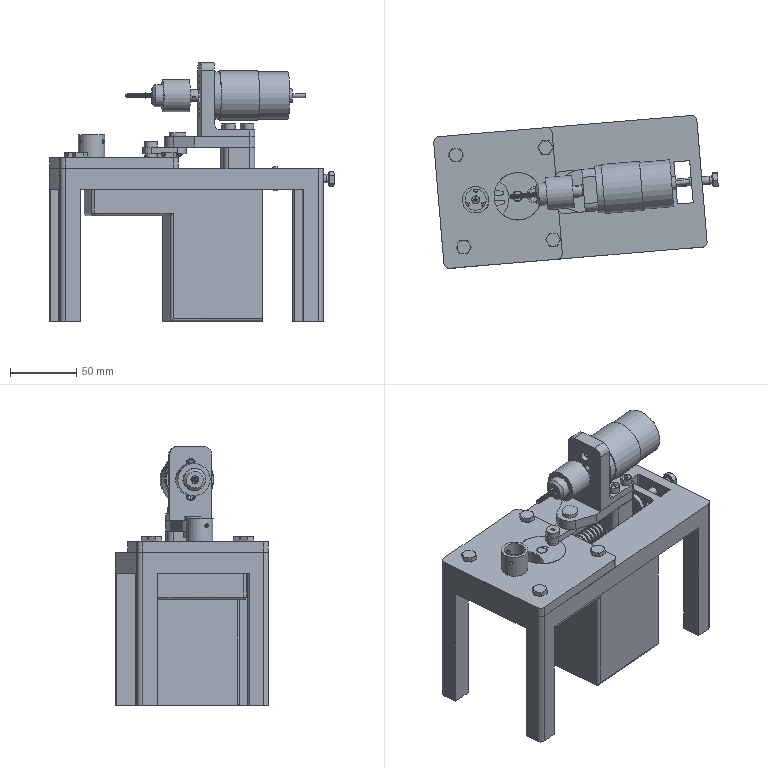Part | NX | features BREP 72, DATUM_CSYS 56, META 40, EXTRUDE 29, SKETCH 21, BLEND 6, CYLINDER 2, FSET 2, SHELL 1, UNITE 1 | 50 solids | 1285 faces | box 215.544 x 115.774 x 196 mm | volume 881623 mm3 | plane 510 | cylinder 389 | spline 210 | cone 120 | torus 54 | sphere 2 | commonest cylinder face diameters 8 x55 52.5 x40 3 x37 2 x30 6 x26 4 x21